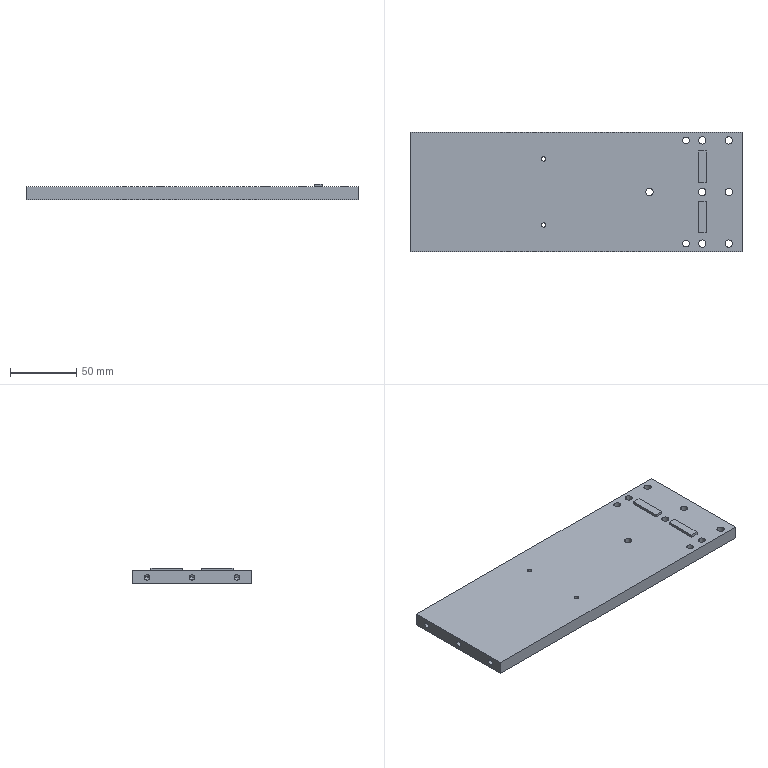Part | 1 solid | 53 faces | box 251 x 90 x 12 mm | volume 223203 mm3 | cylinder 30 | plane 17 | cone 6 | commonest cylinder face diameters 5.5 x14 4.2 x6 3.3 x4 5 x4 10 x2